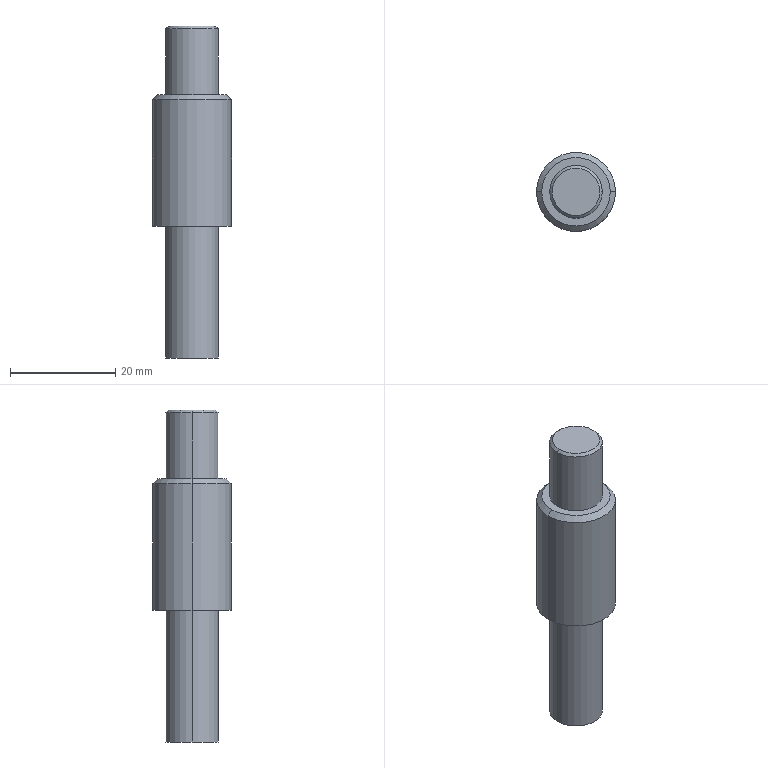Part | SolidWorks | features ICE 3, Chamfer 2, Extrusion 1 | 1 solid | 14 faces | box 15 x 15 x 63 mm | volume 7376 mm3 | cylinder 6 | cone 4 | plane 4 | commonest cylinder face diameters 10 x4 15 x2
STEP:
#1=CARTESIAN_POINT('',(4.5,0.,63.));
#2=VERTEX_POINT('',#1);
#3=CARTESIAN_POINT('',(-4.5,0.,63.));
#4=VERTEX_POINT('',#3);
#5=CARTESIAN_POINT('',(0.,0.,63.));
#6=DIRECTION('',(0.,0.,1.));
#7=DIRECTION('',(1.,0.,0.));
#8=AXIS2_PLACEMENT_3D('',#5,#6,#7);
#9=CIRCLE('',#8,4.5);
#10=EDGE_CURVE('',#2,#4,#9,.T.);
#11=ORIENTED_EDGE('',*,*,#10,.F.);
#12=CARTESIAN_POINT('',(5.,0.,62.5));
#13=VERTEX_POINT('',#12);
#14=CARTESIAN_POINT('',(4.5,0.,63.));
#15=DIRECTION('',(0.7071,0.,-0.7071));
#16=VECTOR('',#15,1000.);
#17=LINE('',#14,#16);
#18=EDGE_CURVE('',#2,#13,#17,.T.);
#19=ORIENTED_EDGE('',*,*,#18,.T.);
#20=CARTESIAN_POINT('',(-5.,0.,62.5));
#21=VERTEX_POINT('',#20);
#22=CARTESIAN_POINT('',(0.,0.,62.5));
#23=DIRECTION('',(0.,0.,-1.));
#24=DIRECTION('',(1.,0.,0.));
#25=AXIS2_PLACEMENT_3D('',#22,#23,#24);
#26=CIRCLE('',#25,5.);
#27=EDGE_CURVE('',#21,#13,#26,.T.);
#28=ORIENTED_EDGE('',*,*,#27,.F.);
#29=CARTESIAN_POINT('',(-4.5,0.,63.));
#30=DIRECTION('',(-0.7071,0.,-0.7071));
#31=VECTOR('',#30,1000.);
#32=LINE('',#29,#31);
#33=EDGE_CURVE('',#4,#21,#32,.T.);
#34=ORIENTED_EDGE('',*,*,#33,.F.);
#35=EDGE_LOOP('',(#11,#19,#28,#34));
#36=FACE_OUTER_BOUND('',#35,.T.);
#37=CARTESIAN_POINT('',(0.,0.,63.));
#38=DIRECTION('',(0.,0.,-1.));
#39=DIRECTION('',(-1.,0.,0.));
#40=AXIS2_PLACEMENT_3D('',#37,#38,#39);
#41=CONICAL_SURFACE('',#40,4.5,0.7854);
#42=ADVANCED_FACE('',(#36),#41,.T.);
#43=CARTESIAN_POINT('',(6.5,0.,50.));
#44=VERTEX_POINT('',#43);
#45=CARTESIAN_POINT('',(-6.5,0.,50.));
#46=VERTEX_POINT('',#45);
#47=CARTESIAN_POINT('',(0.,0.,50.));
#48=DIRECTION('',(0.,0.,1.));
#49=DIRECTION('',(1.,0.,0.));
#50=AXIS2_PLACEMENT_3D('',#47,#48,#49);
#51=CIRCLE('',#50,6.5);
#52=EDGE_CURVE('',#44,#46,#51,.T.);
#53=ORIENTED_EDGE('',*,*,#52,.F.);
#54=CARTESIAN_POINT('',(7.5,0.,49.));
#55=VERTEX_POINT('',#54);
#56=CARTESIAN_POINT('',(6.5,0.,50.));
#57=DIRECTION('',(0.7071,0.,-0.7071));
#58=VECTOR('',#57,1000.);
#59=LINE('',#56,#58);
#60=EDGE_CURVE('',#44,#55,#59,.T.);
#61=ORIENTED_EDGE('',*,*,#60,.T.);
#62=CARTESIAN_POINT('',(-7.5,0.,49.));
#63=VERTEX_POINT('',#62);
#64=CARTESIAN_POINT('',(0.,0.,49.));
#65=DIRECTION('',(0.,0.,-1.));
#66=DIRECTION('',(1.,0.,0.));
#67=AXIS2_PLACEMENT_3D('',#64,#65,#66);
#68=CIRCLE('',#67,7.5);
#69=EDGE_CURVE('',#63,#55,#68,.T.);
#70=ORIENTED_EDGE('',*,*,#69,.F.);
#71=CARTESIAN_POINT('',(-6.5,0.,50.));
#72=DIRECTION('',(-0.7071,0.,-0.7071));
#73=VECTOR('',#72,1000.);
#74=LINE('',#71,#73);
#75=EDGE_CURVE('',#46,#63,#74,.T.);
#76=ORIENTED_EDGE('',*,*,#75,.F.);
#77=EDGE_LOOP('',(#53,#61,#70,#76));
#78=FACE_OUTER_BOUND('',#77,.T.);
#79=CARTESIAN_POINT('',(0.,0.,50.));
#80=DIRECTION('',(0.,0.,-1.));
#81=DIRECTION('',(-1.,0.,0.));
#82=AXIS2_PLACEMENT_3D('',#79,#80,#81);
#83=CONICAL_SURFACE('',#82,6.5,0.7854);
#84=ADVANCED_FACE('',(#78),#83,.T.);
#85=ORIENTED_EDGE('',*,*,#27,.T.);
#86=CARTESIAN_POINT('',(5.,0.,50.));
#87=VERTEX_POINT('',#86);
#88=CARTESIAN_POINT('',(5.,0.,63.));
#89=DIRECTION('',(0.,0.,-1.));
#90=VECTOR('',#89,1000.);
#91=LINE('',#88,#90);
#92=EDGE_CURVE('',#13,#87,#91,.T.);
#93=ORIENTED_EDGE('',*,*,#92,.T.);
#94=CARTESIAN_POINT('',(-5.,0.,50.));
#95=VERTEX_POINT('',#94);
#96=CARTESIAN_POINT('',(0.,0.,50.));
#97=DIRECTION('',(0.,0.,1.));
#98=DIRECTION('',(1.,0.,0.));
#99=AXIS2_PLACEMENT_3D('',#96,#97,#98);
#100=CIRCLE('',#99,5.);
#101=EDGE_CURVE('',#87,#95,#100,.T.);
#102=ORIENTED_EDGE('',*,*,#101,.T.);
#103=CARTESIAN_POINT('',(-5.,0.,63.));
#104=DIRECTION('',(0.,0.,-1.));
#105=VECTOR('',#104,1000.);
#106=LINE('',#103,#105);
#107=EDGE_CURVE('',#21,#95,#106,.T.);
#108=ORIENTED_EDGE('',*,*,#107,.F.);
#109=EDGE_LOOP('',(#85,#93,#102,#108));
#110=FACE_OUTER_BOUND('',#109,.T.);
#111=CARTESIAN_POINT('',(0.,0.,63.));
#112=DIRECTION('',(0.,0.,-1.));
#113=DIRECTION('',(-1.,0.,0.));
#114=AXIS2_PLACEMENT_3D('',#111,#112,#113);
#115=CYLINDRICAL_SURFACE('',#114,5.);
#116=ADVANCED_FACE('',(#110),#115,.T.);
#117=ORIENTED_EDGE('',*,*,#69,.T.);
#118=CARTESIAN_POINT('',(7.5,0.,25.));
#119=VERTEX_POINT('',#118);
#120=CARTESIAN_POINT('',(7.5,0.,33.));
#121=DIRECTION('',(0.,0.,-1.));
#122=VECTOR('',#121,1000.);
#123=LINE('',#120,#122);
#124=EDGE_CURVE('',#55,#119,#123,.T.);
#125=ORIENTED_EDGE('',*,*,#124,.T.);
#126=CARTESIAN_POINT('',(-7.5,0.,25.));
#127=VERTEX_POINT('',#126);
#128=CARTESIAN_POINT('',(0.,0.,25.));
#129=DIRECTION('',(0.,0.,1.));
#130=DIRECTION('',(1.,0.,0.));
#131=AXIS2_PLACEMENT_3D('',#128,#129,#130);
#132=CIRCLE('',#131,7.5);
#133=EDGE_CURVE('',#119,#127,#132,.T.);
#134=ORIENTED_EDGE('',*,*,#133,.T.);
#135=CARTESIAN_POINT('',(-7.5,0.,33.));
#136=DIRECTION('',(0.,0.,-1.));
#137=VECTOR('',#136,1000.);
#138=LINE('',#135,#137);
#139=EDGE_CURVE('',#63,#127,#138,.T.);
#140=ORIENTED_EDGE('',*,*,#139,.F.);
#141=EDGE_LOOP('',(#117,#125,#134,#140));
#142=FACE_OUTER_BOUND('',#141,.T.);
#143=CARTESIAN_POINT('',(0.,0.,33.));
#144=DIRECTION('',(0.,0.,-1.));
#145=DIRECTION('',(-1.,0.,0.));
#146=AXIS2_PLACEMENT_3D('',#143,#144,#145);
#147=CYLINDRICAL_SURFACE('',#146,7.5);
#148=ADVANCED_FACE('',(#142),#147,.T.);
#149=CARTESIAN_POINT('',(5.,0.,25.));
#150=VERTEX_POINT('',#149);
#151=CARTESIAN_POINT('',(-5.,0.,25.));
#152=VERTEX_POINT('',#151);
#153=CARTESIAN_POINT('',(0.,0.,25.));
#154=DIRECTION('',(0.,0.,1.));
#155=DIRECTION('',(1.,0.,0.));
#156=AXIS2_PLACEMENT_3D('',#153,#154,#155);
#157=CIRCLE('',#156,5.);
#158=EDGE_CURVE('',#150,#152,#157,.T.);
#159=ORIENTED_EDGE('',*,*,#158,.F.);
#160=CARTESIAN_POINT('',(5.,0.,0.));
#161=VERTEX_POINT('',#160);
#162=CARTESIAN_POINT('',(5.,0.,25.));
#163=DIRECTION('',(0.,0.,-1.));
#164=VECTOR('',#163,1000.);
#165=LINE('',#162,#164);
#166=EDGE_CURVE('',#150,#161,#165,.T.);
#167=ORIENTED_EDGE('',*,*,#166,.T.);
#168=CARTESIAN_POINT('',(-5.,0.,0.));
#169=VERTEX_POINT('',#168);
#170=CARTESIAN_POINT('',(0.,0.,0.));
#171=DIRECTION('',(0.,0.,1.));
#172=DIRECTION('',(1.,0.,0.));
#173=AXIS2_PLACEMENT_3D('',#170,#171,#172);
#174=CIRCLE('',#173,5.);
#175=EDGE_CURVE('',#161,#169,#174,.T.);
#176=ORIENTED_EDGE('',*,*,#175,.T.);
#177=CARTESIAN_POINT('',(-5.,0.,25.));
#178=DIRECTION('',(0.,0.,-1.));
#179=VECTOR('',#178,1000.);
#180=LINE('',#177,#179);
#181=EDGE_CURVE('',#152,#169,#180,.T.);
#182=ORIENTED_EDGE('',*,*,#181,.F.);
#183=EDGE_LOOP('',(#159,#167,#176,#182));
#184=FACE_OUTER_BOUND('',#183,.T.);
#185=CARTESIAN_POINT('',(0.,0.,25.));
#186=DIRECTION('',(0.,0.,-1.));
#187=DIRECTION('',(-1.,0.,0.));
#188=AXIS2_PLACEMENT_3D('',#185,#186,#187);
#189=CYLINDRICAL_SURFACE('',#188,5.);
#190=ADVANCED_FACE('',(#184),#189,.T.);
#191=ORIENTED_EDGE('',*,*,#166,.F.);
#192=CARTESIAN_POINT('',(0.,0.,25.));
#193=DIRECTION('',(0.,0.,1.));
#194=DIRECTION('',(1.,0.,0.));
#195=AXIS2_PLACEMENT_3D('',#192,#193,#194);
#196=CIRCLE('',#195,5.);
#197=EDGE_CURVE('',#152,#150,#196,.T.);
#198=ORIENTED_EDGE('',*,*,#197,.F.);
#199=ORIENTED_EDGE('',*,*,#181,.T.);
#200=CARTESIAN_POINT('',(0.,0.,0.));
#201=DIRECTION('',(0.,0.,1.));
#202=DIRECTION('',(1.,0.,0.));
#203=AXIS2_PLACEMENT_3D('',#200,#201,#202);
#204=CIRCLE('',#203,5.);
#205=EDGE_CURVE('',#169,#161,#204,.T.);
#206=ORIENTED_EDGE('',*,*,#205,.T.);
#207=EDGE_LOOP('',(#191,#198,#199,#206));
#208=FACE_OUTER_BOUND('',#207,.T.);
#209=CARTESIAN_POINT('',(0.,0.,25.));
#210=DIRECTION('',(0.,0.,-1.));
#211=DIRECTION('',(-1.,0.,0.));
#212=AXIS2_PLACEMENT_3D('',#209,#210,#211);
#213=CYLINDRICAL_SURFACE('',#212,5.);
#214=ADVANCED_FACE('',(#208),#213,.T.);
#215=ORIENTED_EDGE('',*,*,#205,.F.);
#216=ORIENTED_EDGE('',*,*,#175,.F.);
#217=EDGE_LOOP('',(#215,#216));
#218=FACE_OUTER_BOUND('',#217,.T.);
#219=CARTESIAN_POINT('',(0.,0.,0.));
#220=DIRECTION('',(0.,0.,1.));
#221=DIRECTION('',(1.,0.,0.));
#222=AXIS2_PLACEMENT_3D('',#219,#220,#221);
#223=PLANE('',#222);
#224=ADVANCED_FACE('',(#218),#223,.F.);
#225=CARTESIAN_POINT('',(0.,0.,25.));
#226=DIRECTION('',(0.,0.,1.));
#227=DIRECTION('',(1.,0.,0.));
#228=AXIS2_PLACEMENT_3D('',#225,#226,#227);
#229=CIRCLE('',#228,7.5);
#230=EDGE_CURVE('',#127,#119,#229,.T.);
#231=ORIENTED_EDGE('',*,*,#230,.F.);
#232=ORIENTED_EDGE('',*,*,#133,.F.);
#233=EDGE_LOOP('',(#231,#232));
#234=FACE_OUTER_BOUND('',#233,.T.);
#235=ORIENTED_EDGE('',*,*,#197,.T.);
#236=ORIENTED_EDGE('',*,*,#158,.T.);
#237=EDGE_LOOP('',(#235,#236));
#238=FACE_BOUND('',#237,.T.);
#239=CARTESIAN_POINT('',(0.,0.,25.));
#240=DIRECTION('',(0.,0.,1.));
#241=DIRECTION('',(1.,0.,0.));
#242=AXIS2_PLACEMENT_3D('',#239,#240,#241);
#243=PLANE('',#242);
#244=ADVANCED_FACE('',(#234,#238),#243,.F.);
#245=ORIENTED_EDGE('',*,*,#124,.F.);
#246=CARTESIAN_POINT('',(0.,0.,49.));
#247=DIRECTION('',(0.,0.,-1.));
#248=DIRECTION('',(1.,0.,0.));
#249=AXIS2_PLACEMENT_3D('',#246,#247,#248);
#250=CIRCLE('',#249,7.5);
#251=EDGE_CURVE('',#55,#63,#250,.T.);
#252=ORIENTED_EDGE('',*,*,#251,.T.);
#253=ORIENTED_EDGE('',*,*,#139,.T.);
#254=ORIENTED_EDGE('',*,*,#230,.T.);
#255=EDGE_LOOP('',(#245,#252,#253,#254));
#256=FACE_OUTER_BOUND('',#255,.T.);
#257=CARTESIAN_POINT('',(0.,0.,33.));
#258=DIRECTION('',(0.,0.,-1.));
#259=DIRECTION('',(-1.,0.,0.));
#260=AXIS2_PLACEMENT_3D('',#257,#258,#259);
#261=CYLINDRICAL_SURFACE('',#260,7.5);
#262=ADVANCED_FACE('',(#256),#261,.T.);
#263=CARTESIAN_POINT('',(0.,0.,50.));
#264=DIRECTION('',(0.,0.,1.));
#265=DIRECTION('',(1.,0.,0.));
#266=AXIS2_PLACEMENT_3D('',#263,#264,#265);
#267=CIRCLE('',#266,6.5);
#268=EDGE_CURVE('',#46,#44,#267,.T.);
#269=ORIENTED_EDGE('',*,*,#268,.T.);
#270=ORIENTED_EDGE('',*,*,#52,.T.);
#271=EDGE_LOOP('',(#269,#270));
#272=FACE_OUTER_BOUND('',#271,.T.);
#273=CARTESIAN_POINT('',(0.,0.,50.));
#274=DIRECTION('',(0.,0.,1.));
#275=DIRECTION('',(1.,0.,0.));
#276=AXIS2_PLACEMENT_3D('',#273,#274,#275);
#277=CIRCLE('',#276,5.);
#278=EDGE_CURVE('',#95,#87,#277,.T.);
#279=ORIENTED_EDGE('',*,*,#278,.F.);
#280=ORIENTED_EDGE('',*,*,#101,.F.);
#281=EDGE_LOOP('',(#279,#280));
#282=FACE_BOUND('',#281,.T.);
#283=CARTESIAN_POINT('',(0.,0.,50.));
#284=DIRECTION('',(0.,0.,1.));
#285=DIRECTION('',(1.,0.,0.));
#286=AXIS2_PLACEMENT_3D('',#283,#284,#285);
#287=PLANE('',#286);
#288=ADVANCED_FACE('',(#272,#282),#287,.T.);
#289=CARTESIAN_POINT('',(0.,0.,63.));
#290=DIRECTION('',(0.,0.,1.));
#291=DIRECTION('',(1.,0.,0.));
#292=AXIS2_PLACEMENT_3D('',#289,#290,#291);
#293=CIRCLE('',#292,4.5);
#294=EDGE_CURVE('',#4,#2,#293,.T.);
#295=ORIENTED_EDGE('',*,*,#294,.T.);
#296=ORIENTED_EDGE('',*,*,#10,.T.);
#297=EDGE_LOOP('',(#295,#296));
#298=FACE_OUTER_BOUND('',#297,.T.);
#299=CARTESIAN_POINT('',(0.,0.,63.));
#300=DIRECTION('',(0.,0.,1.));
#301=DIRECTION('',(1.,0.,0.));
#302=AXIS2_PLACEMENT_3D('',#299,#300,#301);
#303=PLANE('',#302);
#304=ADVANCED_FACE('',(#298),#303,.T.);
#305=ORIENTED_EDGE('',*,*,#92,.F.);
#306=CARTESIAN_POINT('',(0.,0.,62.5));
#307=DIRECTION('',(0.,0.,-1.));
#308=DIRECTION('',(1.,0.,0.));
#309=AXIS2_PLACEMENT_3D('',#306,#307,#308);
#310=CIRCLE('',#309,5.);
#311=EDGE_CURVE('',#13,#21,#310,.T.);
#312=ORIENTED_EDGE('',*,*,#311,.T.);
#313=ORIENTED_EDGE('',*,*,#107,.T.);
#314=ORIENTED_EDGE('',*,*,#278,.T.);
#315=EDGE_LOOP('',(#305,#312,#313,#314));
#316=FACE_OUTER_BOUND('',#315,.T.);
#317=CARTESIAN_POINT('',(0.,0.,63.));
#318=DIRECTION('',(0.,0.,-1.));
#319=DIRECTION('',(-1.,0.,0.));
#320=AXIS2_PLACEMENT_3D('',#317,#318,#319);
#321=CYLINDRICAL_SURFACE('',#320,5.);
#322=ADVANCED_FACE('',(#316),#321,.T.);
#323=ORIENTED_EDGE('',*,*,#60,.F.);
#324=ORIENTED_EDGE('',*,*,#268,.F.);
#325=ORIENTED_EDGE('',*,*,#75,.T.);
#326=ORIENTED_EDGE('',*,*,#251,.F.);
#327=EDGE_LOOP('',(#323,#324,#325,#326));
#328=FACE_OUTER_BOUND('',#327,.T.);
#329=CARTESIAN_POINT('',(0.,0.,50.));
#330=DIRECTION('',(0.,0.,-1.));
#331=DIRECTION('',(-1.,0.,0.));
#332=AXIS2_PLACEMENT_3D('',#329,#330,#331);
#333=CONICAL_SURFACE('',#332,6.5,0.7854);
#334=ADVANCED_FACE('',(#328),#333,.T.);
#335=ORIENTED_EDGE('',*,*,#18,.F.);
#336=ORIENTED_EDGE('',*,*,#294,.F.);
#337=ORIENTED_EDGE('',*,*,#33,.T.);
#338=ORIENTED_EDGE('',*,*,#311,.F.);
#339=EDGE_LOOP('',(#335,#336,#337,#338));
#340=FACE_OUTER_BOUND('',#339,.T.);
#341=CARTESIAN_POINT('',(0.,0.,63.));
#342=DIRECTION('',(0.,0.,-1.));
#343=DIRECTION('',(-1.,0.,0.));
#344=AXIS2_PLACEMENT_3D('',#341,#342,#343);
#345=CONICAL_SURFACE('',#344,4.5,0.7854);
#346=ADVANCED_FACE('',(#340),#345,.T.);
#347=CLOSED_SHELL('',(#42,#84,#116,#148,#190,#214,#224,#244,#262,#288,#304,#322,#334,#346));
#348=MANIFOLD_SOLID_BREP('',#347);
#349=CARTESIAN_POINT('',(0.,0.,0.));
#350=DIRECTION('',(0.,0.,1.));
#351=DIRECTION('',(1.,0.,0.));
#352=AXIS2_PLACEMENT_3D('',#349,#350,#351);
#353=(LENGTH_UNIT()NAMED_UNIT(*)SI_UNIT(.MILLI.,.METRE.));
#354=UNCERTAINTY_MEASURE_WITH_UNIT(LENGTH_MEASURE(0.00001),#353,'','');
#355=(NAMED_UNIT(*)PLANE_ANGLE_UNIT()SI_UNIT($,.RADIAN.));
#356=(NAMED_UNIT(*)SI_UNIT($,.STERADIAN.)SOLID_ANGLE_UNIT());
#357=(GEOMETRIC_REPRESENTATION_CONTEXT(3)GLOBAL_UNCERTAINTY_ASSIGNED_CONTEXT((#354))GLOBAL_UNIT_ASSIGNED_CONTEXT((#353,#355,#356))REPRESENTATION_CONTEXT('',''));
#358=ADVANCED_BREP_SHAPE_REPRESENTATION('',(#348,#352),#357);